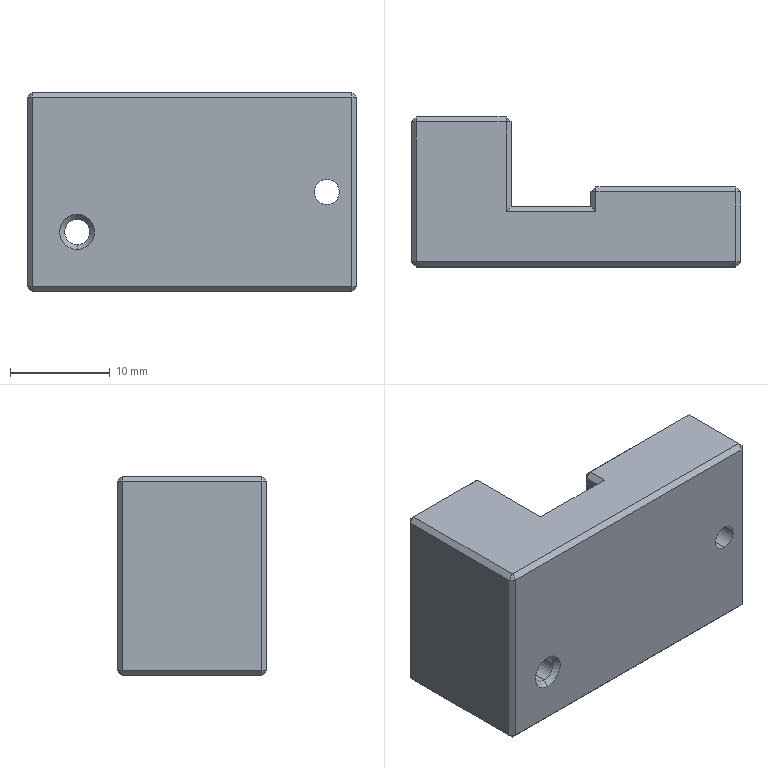Part | NX | features BREP 1 | 1 solid | 67 faces | box 33 x 15 x 20 mm | volume 5682 mm3 | plane 45 | cylinder 12 | cone 10 | commonest cylinder face diameters 2.5 x4 3.3 x4 4 x2 8 x2